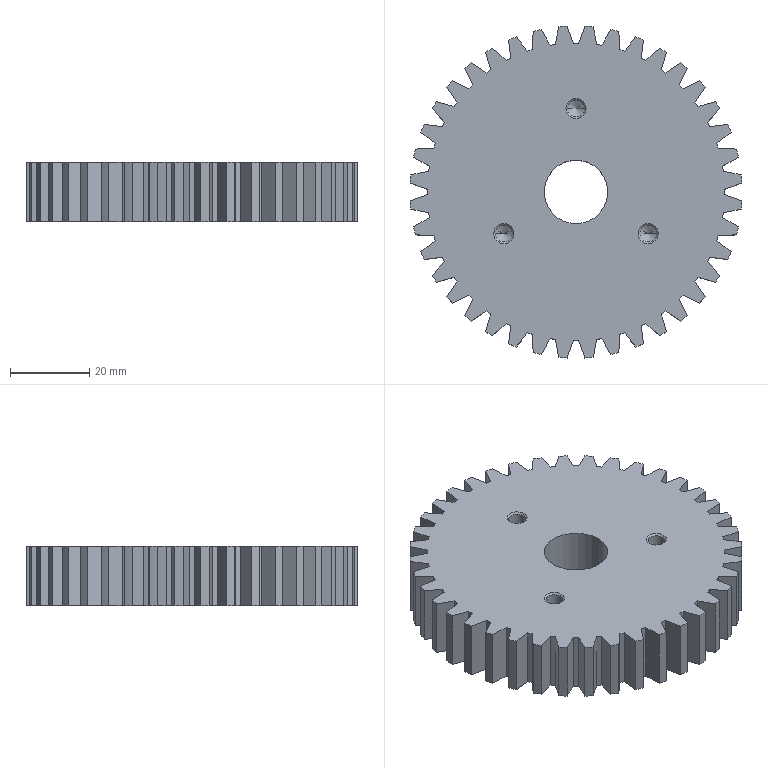Part | SolidWorks | features CirPattern 1, Extrusion 1, HoleWzd 1, ICE 1 | 1 solid | 182 faces | box 83.602 x 83.602 x 15 mm | volume 71569 mm3 | plane 122 | cylinder 48 | cone 12 | commonest cylinder face diameters 83.72 x40 4.2 x6 16 x2